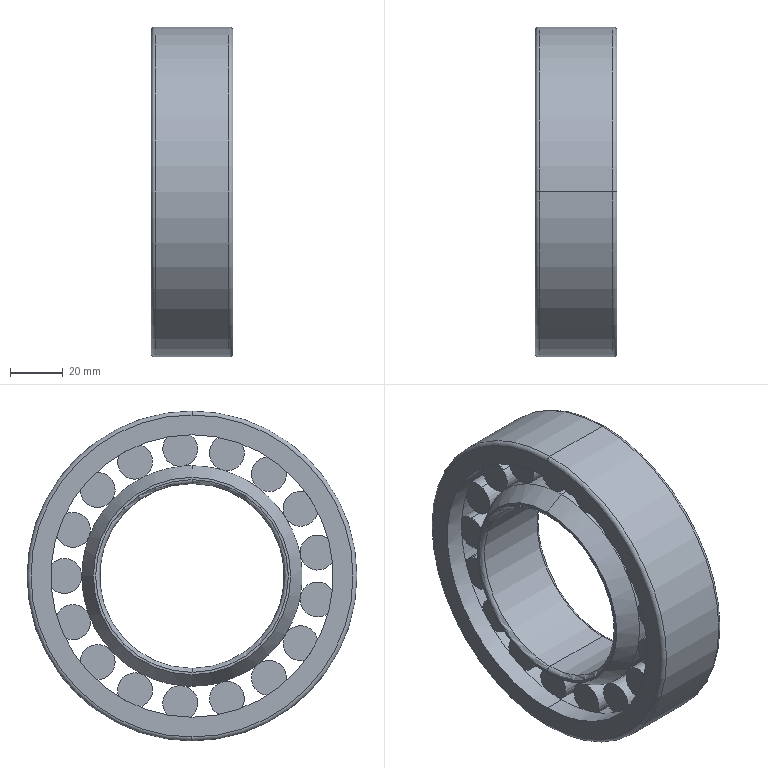Part | SolidWorks | features Revolution 3, CirPattern 1 | 1 solid | 179 faces | box 31 x 125 x 125 mm | volume 173586 mm3 | cylinder 95 | plane 72 | torus 8 | cone 4 | commonest cylinder face diameters 13.25 x51 83.5 x18 110 x18 107 x4 70 x2 125 x2